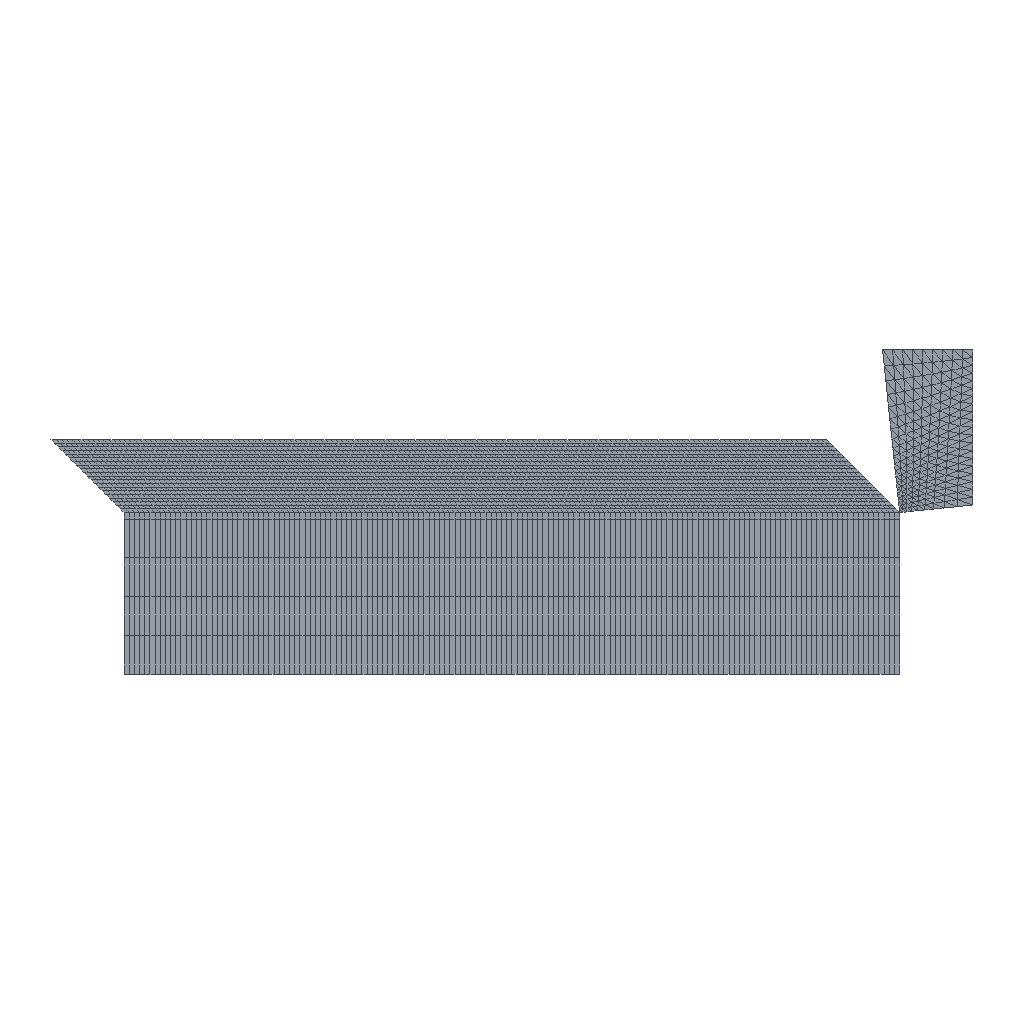Simulation study | abaqus
Set-up summary:
category,name,step,type,value,unit,region
solver,abaqus
solver,version,,,Abaqus/Explicit 2020
units,not stated in the deck,,not stated
analysis,deck,,dynamic temperature-displacement,dynamic temperature-displacement
load_step,Step-1,Step-1,dynamic temperature-displacement
load_step,requested,,,1
mesh,nodes,,,4136
mesh,elements,,,4110
element_type,CPE3T,,plane,360
element_type,CPE4RT,,plane,3750
load,load commands in deck,,count,1
bc,support commands in deck,,count,4
material,TI,,in results
material,TI-COPY,,in results
material,TI6AL4V-GAI,,in results
material,TI6AL4V-SUN,,in results
material,YG6,,in results
check,setup vs results,,match,"per instance, exact: element labels, types and connectivity; labels of the nodes the elements use; coordinates of those nodes at SINGLE_PRECISION in 2 of 2 instance(s)"
Abaqus input file, long lists of numbers shortened:
*Heading
** Job name: Job-3 Model name: Model-1-Copy-Copy
** Generated by: Abaqus/CAE 2020
*Preprint, echo=NO, model=NO, history=NO, contact=NO
**
** PARTS
**
*Part, name=Part-tool
*Node
      1, 0.05,  0.3
      2, 0.05659,  0.2373
** (208 more lines like these left out)
*Element, type=CPE3T
  1,   1,   2,  23
  2,  23,  22,   1
** (358 more lines like these left out)
*Nset, nset=Set-6, generate
   1,  210,    1
*Elset, elset=Set-6, generate
   1,  360,    1
** Section: Section-tool
*Solid Section, elset=Set-6, material=YG6
2.5,
*End Part
**
*Part, name=work
*Node
      1,          1.5, -0.2125
      2,         -1.5, -0.2125
** (3924 more lines like these left out)
*Element, type=CPE4RT
  1,    1,    9,  649,  312
  2,    9,   10,  650,  649
** (3748 more lines like these left out)
*Nset, nset=Set-4, generate
    1,  3926,     1
*Elset, elset=Set-4, generate
    1,  3750,     1
*Nset, nset=Set-12, generate
    1,  3926,     1
*Elset, elset=Set-12
    1,    2,    3,    4,    5,    6,    7,    8,    9,   10,   11,   12,   13,   14,   15,   16
   17,   18,   19,   20,   21,   22,   23,   24,   25,   26,   27,   28,   29,   30,   31,   32
** (223 more lines like these left out)
*Nset, nset=Set-13
   1,   2,   5,   6,   9,  10,  11,  12,  13,  14,  15,  16,  17,  18,  19,  20
  21,  22,  23,  24,  25,  26,  27,  28,  29,  30,  31,  32,  33,  34,  35,  36
** (17 more lines like these left out)
*Elset, elset=Set-13, generate
 601,  750,    1
** Section: ti
*Solid Section, elset=Set-12, material=ti
,
** Section: middle
*Solid Section, elset=Set-13, material=ti-Copy
,
*End Part
**
**
** ASSEMBLY
**
*Assembly, name=Assembly
**
*Instance, name=Part-tool-1, part=Part-tool
    1.384,     0.1423,           0.
*End Instance
**
*Instance, name=work-1, part=work
*End Instance
**
*Node
      1,   1.784,   0.4423,           0.
*Nset, nset=Set-9, instance=work-1, generate
    1,  3926,     1
*Elset, elset=Set-9, instance=work-1, generate
    1,  3750,     1
*Nset, nset=Set-10, instance=Part-tool-1, generate
   1,  210,    1
*Elset, elset=Set-10, instance=Part-tool-1, generate
   1,  360,    1
*Nset, nset=Set-11, instance=work-1
   2,   3,   4, 158, 159, 160, 161, 162, 163, 164, 165, 166, 167, 168, 169, 170
 171, 172, 173, 174, 175, 176, 177, 178, 179, 180, 181, 182, 183, 184, 185, 186
** (8 more lines like these left out)
*Elset, elset=Set-11, instance=work-1
 150, 300, 450, 451, 452, 453, 454, 455, 456, 457, 458, 459, 460, 461, 462, 463
 464, 465, 466, 467, 468, 469, 470, 471, 472, 473, 474, 475, 476, 477, 478, 479
** (8 more lines like these left out)
*Nset, nset=Set-RP
 1,
*Nset, nset=b_Set-7, instance=Part-tool-1, generate
   1,  210,    1
*Elset, elset=b_Set-7, instance=Part-tool-1, generate
   1,  360,    1
*Nset, nset=s_Set-12, instance=work-1
    1,    2,    5,    6,    7,    8,    9,   10,   11,   12,   13,   14,   15,   16,   17,   18
   19,   20,   21,   22,   23,   24,   25,   26,   27,   28,   29,   30,   31,   32,   33,   34
** (206 more lines like these left out)
*Elset, elset=s_Set-12, instance=work-1, generate
  601,  3750,     1
*Nset, nset=s_Set-13, instance=work-1
    1,    2,    5,    6,    7,    8,    9,   10,   11,   12,   13,   14,   15,   16,   17,   18
   19,   20,   21,   22,   23,   24,   25,   26,   27,   28,   29,   30,   31,   32,   33,   34
** (206 more lines like these left out)
*Elset, elset=s_Set-13, instance=work-1, generate
  601,  3750,     1
*Nset, nset=s_Set-14, instance=work-1
    1,    2,    5,    6,    7,    8,    9,   10,   11,   12,   13,   14,   15,   16,   17,   18
   19,   20,   21,   22,   23,   24,   25,   26,   27,   28,   29,   30,   31,   32,   33,   34
** (206 more lines like these left out)
*Elset, elset=s_Set-14, instance=work-1, generate
  601,  3750,     1
*Nset, nset=_PickedSet38, internal
 1,
*Elset, elset=_Surf-8_S2, internal, instance=work-1, generate
  750,  3750,   150
*Elset, elset=_Surf-8_S1, internal, instance=work-1, generate
 751,  900,    1
*Elset, elset=_Surf-8_S4, internal, instance=work-1, generate
  751,  3601,   150
*Surface, type=ELEMENT, name=Surf-8
_Surf-8_S2, S2
_Surf-8_S1, S1
_Surf-8_S4, S4
*Elset, elset=_Surf-9_S1, internal, instance=work-1, generate
 751,  900,    1
*Elset, elset=_Surf-9_S2, internal, instance=work-1, generate
  900,  3750,   150
*Elset, elset=_Surf-9_S4, internal, instance=work-1, generate
  751,  3601,   150
*Surface, type=ELEMENT, name=Surf-9
_Surf-9_S1, S1
_Surf-9_S2, S2
_Surf-9_S4, S4
*Elset, elset=_m_Surf-7_S1, internal, instance=Part-tool-1, generate
  1,  39,   2
*Elset, elset=_m_Surf-7_S2, internal, instance=Part-tool-1
   2,  39,  42,  79,  82, 119, 122, 159, 162, 199, 202, 239, 242, 279, 282, 319
 322, 359
*Surface, type=ELEMENT, name=m_Surf-7
_m_Surf-7_S1, S1
_m_Surf-7_S2, S2
*Elset, elset=_m_Surf-10_S1, internal, instance=Part-tool-1, generate
  1,  39,   2
*Elset, elset=_m_Surf-10_S2, internal, instance=Part-tool-1
   2,  39,  42,  79,  82, 119, 122, 159, 162, 199, 202, 239, 242, 279, 282, 319
 322, 359
*Surface, type=ELEMENT, name=m_Surf-10
_m_Surf-10_S1, S1
_m_Surf-10_S2, S2
*Elset, elset=_s_Surf-10_S2, internal, instance=work-1, generate
  750,  3750,   150
*Elset, elset=_s_Surf-10_S4, internal, instance=work-1, generate
  601,  3601,   150
*Elset, elset=_s_Surf-10_S1, internal, instance=work-1, generate
 751,  900,    1
*Surface, type=ELEMENT, name=s_Surf-10
_s_Surf-10_S2, S2
_s_Surf-10_S4, S4
_s_Surf-10_S1, S1
** Constraint: Constraint-1
*Rigid Body, ref node=_PickedSet38, elset=b_Set-7, position=CENTER OF MASS
*End Assembly
**
** MATERIALS
**
*Material, name=TI6AL4V-gai
*Conductivity
  5.44, 20.
   6.7,100.
  8.79,200.
 10.47,300.
 12.56,400.
 14.24,500.
 15.49,600.
*Damage Initiation, criterion=JOHNSON COOK
 -0.09,  0.25, -0.48, 0.014,  3.87, 1630.,   25.,    1.
*Damage Evolution, type=DISPLACEMENT
 0.1,
*Density
 4.44e-09,
*Elastic
105000., 0.31
*Expansion
 9.4e-06,100.
 9.5e-06,200.
 9.6e-06,300.
 9.7e-06,400.
 9.9e-06,500.
   1e-05,600.
*Inelastic Heat Fraction
         0.9,
*Plastic, hardening=JOHNSON COOK
875.,  793., 0.386,  0.71, 1630.,   25.
*Rate Dependent, type=JOHNSON COOK
 0.01,1.
*Specific Heat
 5.65e+08, 20.
 6.78e+08,100.
 6.91e+08,200.
 7.03e+08,300.
 7.41e+08,400.
 7.54e+08,500.
 8.79e+08,600.
*Material, name=TI6AL4V-sun
*Conductivity
  5.44, 20.
   6.7,100.
  8.79,200.
 10.47,300.
 12.56,400.
 14.24,500.
 15.49,600.
*Damage Initiation, criterion=JOHNSON COOK
 -0.09,  0.25, -0.48, 0.014,  3.87, 1630.,   25.,    1.
*Damage Evolution, type=DISPLACEMENT
 0.15,
*Density
 4.44e-09,
*Elastic
105000., 0.31
*Expansion
 9.4e-06,100.
 9.5e-06,200.
 9.6e-06,300.
 9.7e-06,400.
 9.9e-06,500.
   1e-05,600.
*Inelastic Heat Fraction
         0.9,
*Plastic, hardening=JOHNSON COOK
875.,  793., 0.386,  0.71, 1630.,   25.
*Rate Dependent, type=JOHNSON COOK
 0.01,1.
*Specific Heat
 5.65e+08, 20.
 6.78e+08,100.
 6.91e+08,200.
 7.03e+08,300.
 7.41e+08,400.
 7.54e+08,500.
 8.79e+08,600.
*Material, name=YG6
*Conductivity
 79.6,
*Density
 1.485e-08,
*Elastic
640000., 0.22
*Expansion
 4.7e-06,
*Inelastic Heat Fraction
         0.9,
*Specific Heat
 1.76e+08,
*Material, name=ti
*Conductivity
  7.5, 20.
  8.7,200.
 11.8,500.
*Damage Initiation, criterion=JOHNSON COOK
 -0.09,  0.25,  -0.5, 0.014,  3.87, 1650.,   25.,    1.
*Damage Evolution, type=DISPLACEMENT
 0.1,
*Density
 4.44e-09,
*Elastic
108000., 0.33
*Expansion
 9.1e-06, 20.
 9.2e-06,250.
 9.7e-06,500.
*Inelastic Heat Fraction
         0.9,
*Plastic, hardening=JOHNSON COOK
860., 683., 0.47,   1.,1650.,  25.
*Rate Dependent, type=JOHNSON COOK
 0.035,1.
*Specific Heat
 5.263e+08,
*Material, name=ti-Copy
*Conductivity
  7.5, 20.
  8.7,200.
 11.8,500.
*Damage Initiation, criterion=JOHNSON COOK
 -0.09,  0.25,  -0.5, 0.014,  3.87, 1650.,   25.,    1.
*Damage Evolution, type=DISPLACEMENT
 0.04,
*Density
 4.44e-09,
*Elastic
108000., 0.33
*Expansion
 9.1e-06, 20.
 9.2e-06,250.
 9.7e-06,500.
*Inelastic Heat Fraction
         0.9,
*Plastic, hardening=JOHNSON COOK
860., 683., 0.47,   1.,1650.,  25.
*Rate Dependent, type=JOHNSON COOK
 0.035,1.
*Specific Heat
 5.263e+08,
**
** INTERACTION PROPERTIES
**
*Surface Interaction, name=IntProp-1
*Friction
 0.1,
*Surface Behavior, pressure-overclosure=HARD
*Surface Interaction, name=zijie
*Friction
 0.5,
*Surface Behavior, pressure-overclosure=HARD
**
** BOUNDARY CONDITIONS
**
** Name: BC-1 Type: 对称/反对称/完全固定
*Boundary
Set-11, ENCASTRE
**
** PREDEFINED FIELDS
**
** Name: Predefined Field-1   Type: Temperature
*Initial Conditions, type=TEMPERATURE
Set-9, 20.
** Name: Predefined Field-2   Type: Temperature
*Initial Conditions, type=TEMPERATURE
Set-10, 20.
** ----------------------------------------------------------------
**
** STEP: Step-1
**
*Step, name=Step-1, nlgeom=YES
*Dynamic Temperature-displacement, Explicit
, 0.001
*Bulk Viscosity
0.06, 1.2
** Mass Scaling: Semi-Automatic
**               Whole Model
*Fixed Mass Scaling, factor=200.
**
** BOUNDARY CONDITIONS
**
** Name: BC-2 Type: 速度/角速度
*Boundary, type=VELOCITY
Set-RP, 1, 1, -1666.
Set-RP, 2, 2
Set-RP, 6, 6
*Adaptive Mesh Controls, name=Ada-1, curvature refinement=5.
0.5, 0., 0.5
**
** INTERACTIONS
**
** Interaction: Int-3
*Contact Pair, interaction=zijie, mechanical constraint=PENALTY, cpset=Int-3
Surf-9,
** Interaction: Int-4
*Contact Pair, interaction=IntProp-1, mechanical constraint=PENALTY, cpset=Int-4
m_Surf-10, s_Surf-10
** Interaction: Int-2
*Contact, op=NEW
*Contact Inclusions, ALL EXTERIOR
*Contact Property Assignment
 ,  , zijie
**
** OUTPUT REQUESTS
**
*Restart, write, number interval=1, time marks=NO
**
** FIELD OUTPUT: F-Output-1
**
*Output, field, number interval=100
*Node Output
A, NT, RF, RFL, U, V
*Element Output, directions=YES
E, EVF, HFL, LE, MISES, PE, PEEQ, PEEQVAVG, PEVAVG, S, STATUS, SVAVG, TEMP
*Contact Output
CSTRESS,
**
** HISTORY OUTPUT: H-Output-1
**
*Output, history, time interval=5e-07
*Node Output, nset=Set-RP
RF1, RF2, RF3
*End Step
Results summary:
result,step,Step-1,partial,increments=86260 time=0.0005915/0.001
result,analysis,,,"dynamic temperature-displacement, explict"
result,last_loadstep,,,1
result,primary field,,,"U, NT11"
result,reaction total,,FX,75.202,model units
result,reaction total,,FY,-45.784,model units
result,reaction total,,FZ,0.0,model units